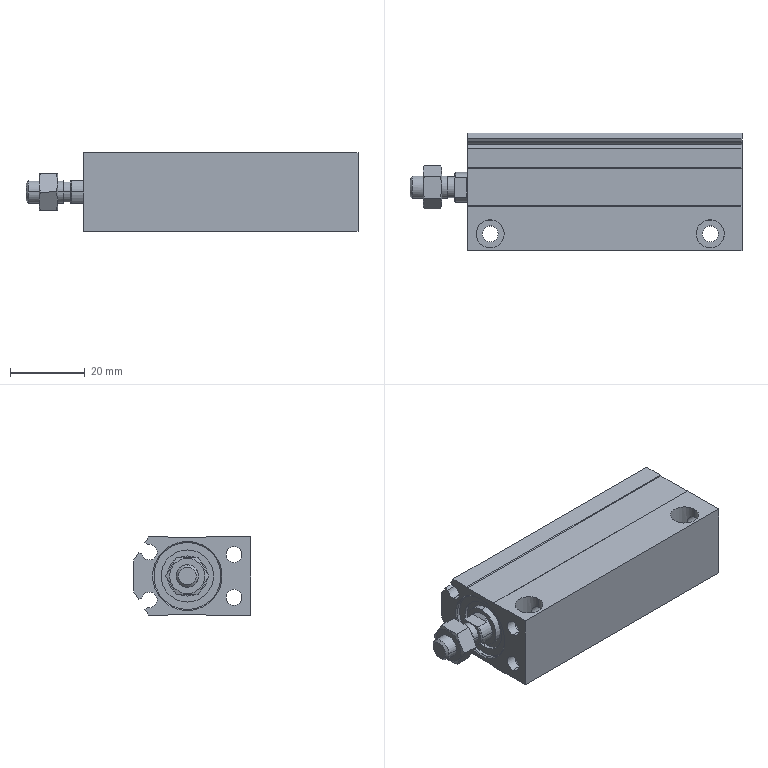Part | SolidWorks | features BaseBody 3 | 3 solids | 123 faces | box 89 x 31.5 x 21 mm | volume 33779 mm3 | cylinder 54 | plane 50 | cone 19 | commonest cylinder face diameters 4.3 x16 7.5 x8 4.2 x6 4.134 x4 8 x4 16 x4